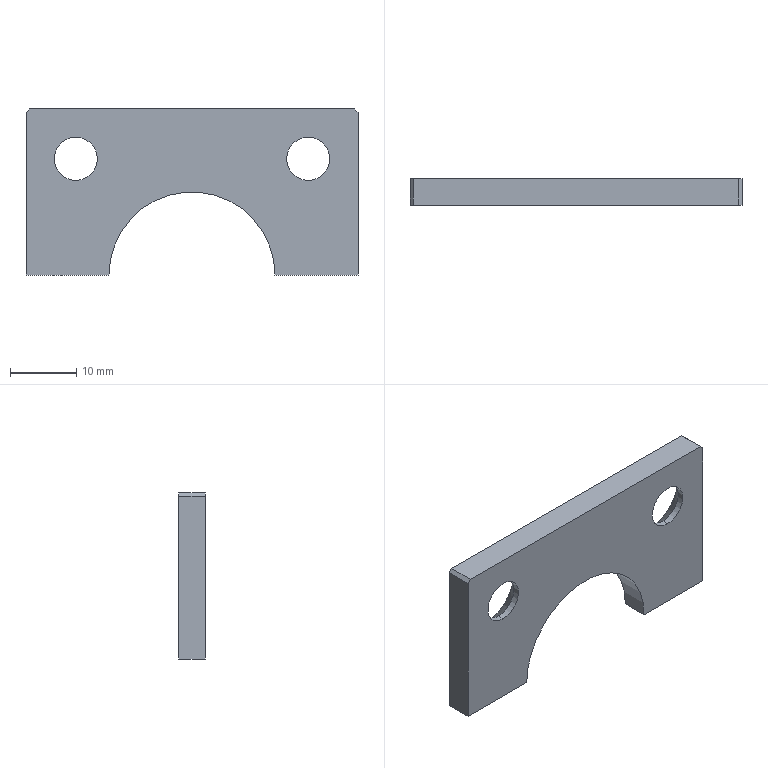Part | STEP file | Cuon T phu H01_4 | 1 solid | 18 faces | box 50 x 4 x 25 mm | volume 3511 mm3 | plane 9 | cylinder 5 | cone 4 | commonest cylinder face diameters 6.5 x4 25 x1
STEP:
#1=CARTESIAN_POINT('',(0.,0.,0.));
#2=DIRECTION('',(0.,0.,1.));
#3=DIRECTION('',(1.,0.,0.));
#4=AXIS2_PLACEMENT_3D('',#1,#2,#3);
#5=CARTESIAN_POINT('',(-17.5,1.,20.75));
#6=VERTEX_POINT('',#5);
#7=CARTESIAN_POINT('',(-17.5,4.,23.75));
#8=VERTEX_POINT('',#7);
#9=CARTESIAN_POINT('',(-17.5,1.,20.75));
#10=DIRECTION('',(0.,0.7071,0.7071));
#11=VECTOR('',#10,1.);
#12=LINE('',#9,#11);
#13=CARTESIAN_POINT('',(-17.5,1.,17.5));
#14=DIRECTION('',(0.,1.,0.));
#15=DIRECTION('',(0.,0.,1.));
#16=AXIS2_PLACEMENT_3D('',#13,#14,#15);
#17=CONICAL_SURFACE('',#16,3.25,0.7854);
#18=CARTESIAN_POINT('',(6.283,0.));
#19=DIRECTION('',(0.,1.));
#20=VECTOR('',#19,1.);
#21=LINE('',#18,#20);
#22=(GEOMETRIC_REPRESENTATION_CONTEXT(2)PARAMETRIC_REPRESENTATION_CONTEXT()REPRESENTATION_CONTEXT('',''));
#23=DEFINITIONAL_REPRESENTATION('',(#21),#22);
#24=PCURVE('',#17,#23);
#25=CARTESIAN_POINT('',(-17.5,1.,17.5));
#26=DIRECTION('',(0.,1.,0.));
#27=DIRECTION('',(0.,0.,1.));
#28=AXIS2_PLACEMENT_3D('',#25,#26,#27);
#29=CONICAL_SURFACE('',#28,3.25,0.7854);
#30=CARTESIAN_POINT('',(0.,0.));
#31=DIRECTION('',(0.,1.));
#32=VECTOR('',#31,1.);
#33=LINE('',#30,#32);
#34=(GEOMETRIC_REPRESENTATION_CONTEXT(2)PARAMETRIC_REPRESENTATION_CONTEXT()REPRESENTATION_CONTEXT('',''));
#35=DEFINITIONAL_REPRESENTATION('',(#33),#34);
#36=PCURVE('',#29,#35);
#37=SURFACE_CURVE('',#12,(#24,#36),.PCURVE_S1.);
#38=EDGE_CURVE('',#6,#8,#37,.T.);
#39=ORIENTED_EDGE('',*,*,#38,.T.);
#40=CARTESIAN_POINT('',(-17.5,4.,11.25));
#41=VERTEX_POINT('',#40);
#42=CARTESIAN_POINT('',(-17.5,4.,17.5));
#43=DIRECTION('',(0.,-1.,0.));
#44=DIRECTION('',(0.,0.,1.));
#45=AXIS2_PLACEMENT_3D('',#42,#43,#44);
#46=CIRCLE('',#45,6.25);
#47=CARTESIAN_POINT('',(6.283,3.));
#48=DIRECTION('',(-1.,0.));
#49=VECTOR('',#48,1.);
#50=LINE('',#47,#49);
#51=(GEOMETRIC_REPRESENTATION_CONTEXT(2)PARAMETRIC_REPRESENTATION_CONTEXT()REPRESENTATION_CONTEXT('',''));
#52=DEFINITIONAL_REPRESENTATION('',(#50),#51);
#53=PCURVE('',#17,#52);
#54=CARTESIAN_POINT('',(0.,4.,0.));
#55=DIRECTION('',(0.,1.,0.));
#56=DIRECTION('',(0.,0.,1.));
#57=AXIS2_PLACEMENT_3D('',#54,#55,#56);
#58=PLANE('',#57);
#59=CARTESIAN_POINT('',(23.75,-17.5));
#60=CARTESIAN_POINT('',(23.75,-28.325));
#61=CARTESIAN_POINT('',(14.375,-22.913));
#62=CARTESIAN_POINT('',(5.,-17.5));
#63=CARTESIAN_POINT('',(14.375,-12.087));
#64=CARTESIAN_POINT('',(23.75,-6.675));
#65=CARTESIAN_POINT('',(23.75,-17.5));
#66=(BOUNDED_CURVE()B_SPLINE_CURVE(2,(#59,#60,#61,#62,#63,#64,#65),.UNSPECIFIED.,.T.,.F.)B_SPLINE_CURVE_WITH_KNOTS((1,2,2,2,2,1),(-2.094,0.,2.094,4.189,6.283,8.378),.UNSPECIFIED.)CURVE()GEOMETRIC_REPRESENTATION_ITEM()RATIONAL_B_SPLINE_CURVE((1.,0.5,1.,0.5,1.,0.5,1.))REPRESENTATION_ITEM(''));
#67=(GEOMETRIC_REPRESENTATION_CONTEXT(2)PARAMETRIC_REPRESENTATION_CONTEXT()REPRESENTATION_CONTEXT('',''));
#68=DEFINITIONAL_REPRESENTATION('',(#66),#67);
#69=PCURVE('',#58,#68);
#70=SURFACE_CURVE('',#46,(#53,#69),.PCURVE_S1.);
#71=EDGE_CURVE('',#8,#41,#70,.T.);
#72=ORIENTED_EDGE('',*,*,#71,.T.);
#73=CARTESIAN_POINT('',(-17.5,1.,14.25));
#74=VERTEX_POINT('',#73);
#75=CARTESIAN_POINT('',(-17.5,1.,14.25));
#76=DIRECTION('',(0.,0.7071,-0.7071));
#77=VECTOR('',#76,1.);
#78=LINE('',#75,#77);
#79=CARTESIAN_POINT('',(3.142,0.));
#80=DIRECTION('',(0.,1.));
#81=VECTOR('',#80,1.);
#82=LINE('',#79,#81);
#83=(GEOMETRIC_REPRESENTATION_CONTEXT(2)PARAMETRIC_REPRESENTATION_CONTEXT()REPRESENTATION_CONTEXT('',''));
#84=DEFINITIONAL_REPRESENTATION('',(#82),#83);
#85=PCURVE('',#17,#84);
#86=CARTESIAN_POINT('',(3.142,0.));
#87=DIRECTION('',(0.,1.));
#88=VECTOR('',#87,1.);
#89=LINE('',#86,#88);
#90=(GEOMETRIC_REPRESENTATION_CONTEXT(2)PARAMETRIC_REPRESENTATION_CONTEXT()REPRESENTATION_CONTEXT('',''));
#91=DEFINITIONAL_REPRESENTATION('',(#89),#90);
#92=PCURVE('',#29,#91);
#93=SURFACE_CURVE('',#78,(#85,#92),.PCURVE_S1.);
#94=EDGE_CURVE('',#74,#41,#93,.T.);
#95=ORIENTED_EDGE('',*,*,#94,.F.);
#96=CARTESIAN_POINT('',(-17.5,1.,17.5));
#97=DIRECTION('',(0.,1.,0.));
#98=DIRECTION('',(0.,0.,1.));
#99=AXIS2_PLACEMENT_3D('',#96,#97,#98);
#100=CIRCLE('',#99,3.25);
#101=CARTESIAN_POINT('',(0.,0.));
#102=DIRECTION('',(1.,0.));
#103=VECTOR('',#102,1.);
#104=LINE('',#101,#103);
#105=(GEOMETRIC_REPRESENTATION_CONTEXT(2)PARAMETRIC_REPRESENTATION_CONTEXT()REPRESENTATION_CONTEXT('',''));
#106=DEFINITIONAL_REPRESENTATION('',(#104),#105);
#107=PCURVE('',#17,#106);
#108=CARTESIAN_POINT('',(-17.5,4.,17.5));
#109=DIRECTION('',(0.,-1.,0.));
#110=DIRECTION('',(0.,0.,-1.));
#111=AXIS2_PLACEMENT_3D('',#108,#109,#110);
#112=CYLINDRICAL_SURFACE('',#111,3.25);
#113=CARTESIAN_POINT('',(9.425,3.));
#114=DIRECTION('',(-1.,0.));
#115=VECTOR('',#114,1.);
#116=LINE('',#113,#115);
#117=(GEOMETRIC_REPRESENTATION_CONTEXT(2)PARAMETRIC_REPRESENTATION_CONTEXT()REPRESENTATION_CONTEXT('',''));
#118=DEFINITIONAL_REPRESENTATION('',(#116),#117);
#119=PCURVE('',#112,#118);
#120=SURFACE_CURVE('',#100,(#107,#119),.PCURVE_S1.);
#121=EDGE_CURVE('',#74,#6,#120,.T.);
#122=ORIENTED_EDGE('',*,*,#121,.T.);
#123=EDGE_LOOP('',(#39,#72,#95,#122));
#124=FACE_BOUND('',#123,.F.);
#125=ADVANCED_FACE('',(#124),#17,.F.);
#126=CARTESIAN_POINT('',(17.5,1.,20.75));
#127=VERTEX_POINT('',#126);
#128=CARTESIAN_POINT('',(17.5,4.,23.75));
#129=VERTEX_POINT('',#128);
#130=CARTESIAN_POINT('',(17.5,1.,20.75));
#131=DIRECTION('',(0.,0.7071,0.7071));
#132=VECTOR('',#131,1.);
#133=LINE('',#130,#132);
#134=CARTESIAN_POINT('',(17.5,1.,17.5));
#135=DIRECTION('',(0.,1.,0.));
#136=DIRECTION('',(0.,0.,1.));
#137=AXIS2_PLACEMENT_3D('',#134,#135,#136);
#138=CONICAL_SURFACE('',#137,3.25,0.7854);
#139=CARTESIAN_POINT('',(6.283,0.));
#140=DIRECTION('',(0.,1.));
#141=VECTOR('',#140,1.);
#142=LINE('',#139,#141);
#143=(GEOMETRIC_REPRESENTATION_CONTEXT(2)PARAMETRIC_REPRESENTATION_CONTEXT()REPRESENTATION_CONTEXT('',''));
#144=DEFINITIONAL_REPRESENTATION('',(#142),#143);
#145=PCURVE('',#138,#144);
#146=CARTESIAN_POINT('',(17.5,1.,17.5));
#147=DIRECTION('',(0.,1.,0.));
#148=DIRECTION('',(0.,0.,1.));
#149=AXIS2_PLACEMENT_3D('',#146,#147,#148);
#150=CONICAL_SURFACE('',#149,3.25,0.7854);
#151=CARTESIAN_POINT('',(0.,0.));
#152=DIRECTION('',(0.,1.));
#153=VECTOR('',#152,1.);
#154=LINE('',#151,#153);
#155=(GEOMETRIC_REPRESENTATION_CONTEXT(2)PARAMETRIC_REPRESENTATION_CONTEXT()REPRESENTATION_CONTEXT('',''));
#156=DEFINITIONAL_REPRESENTATION('',(#154),#155);
#157=PCURVE('',#150,#156);
#158=SURFACE_CURVE('',#133,(#145,#157),.PCURVE_S1.);
#159=EDGE_CURVE('',#127,#129,#158,.T.);
#160=ORIENTED_EDGE('',*,*,#159,.T.);
#161=CARTESIAN_POINT('',(17.5,4.,11.25));
#162=VERTEX_POINT('',#161);
#163=CARTESIAN_POINT('',(17.5,4.,17.5));
#164=DIRECTION('',(0.,-1.,0.));
#165=DIRECTION('',(0.,0.,1.));
#166=AXIS2_PLACEMENT_3D('',#163,#164,#165);
#167=CIRCLE('',#166,6.25);
#168=CARTESIAN_POINT('',(6.283,3.));
#169=DIRECTION('',(-1.,0.));
#170=VECTOR('',#169,1.);
#171=LINE('',#168,#170);
#172=(GEOMETRIC_REPRESENTATION_CONTEXT(2)PARAMETRIC_REPRESENTATION_CONTEXT()REPRESENTATION_CONTEXT('',''));
#173=DEFINITIONAL_REPRESENTATION('',(#171),#172);
#174=PCURVE('',#138,#173);
#175=CARTESIAN_POINT('',(23.75,17.5));
#176=CARTESIAN_POINT('',(23.75,6.675));
#177=CARTESIAN_POINT('',(14.375,12.087));
#178=CARTESIAN_POINT('',(5.,17.5));
#179=CARTESIAN_POINT('',(14.375,22.913));
#180=CARTESIAN_POINT('',(23.75,28.325));
#181=CARTESIAN_POINT('',(23.75,17.5));
#182=(BOUNDED_CURVE()B_SPLINE_CURVE(2,(#175,#176,#177,#178,#179,#180,#181),.UNSPECIFIED.,.T.,.F.)B_SPLINE_CURVE_WITH_KNOTS((1,2,2,2,2,1),(-2.094,0.,2.094,4.189,6.283,8.378),.UNSPECIFIED.)CURVE()GEOMETRIC_REPRESENTATION_ITEM()RATIONAL_B_SPLINE_CURVE((1.,0.5,1.,0.5,1.,0.5,1.))REPRESENTATION_ITEM(''));
#183=(GEOMETRIC_REPRESENTATION_CONTEXT(2)PARAMETRIC_REPRESENTATION_CONTEXT()REPRESENTATION_CONTEXT('',''));
#184=DEFINITIONAL_REPRESENTATION('',(#182),#183);
#185=PCURVE('',#58,#184);
#186=SURFACE_CURVE('',#167,(#174,#185),.PCURVE_S1.);
#187=EDGE_CURVE('',#129,#162,#186,.T.);
#188=ORIENTED_EDGE('',*,*,#187,.T.);
#189=CARTESIAN_POINT('',(17.5,1.,14.25));
#190=VERTEX_POINT('',#189);
#191=CARTESIAN_POINT('',(17.5,1.,14.25));
#192=DIRECTION('',(0.,0.7071,-0.7071));
#193=VECTOR('',#192,1.);
#194=LINE('',#191,#193);
#195=CARTESIAN_POINT('',(3.142,0.));
#196=DIRECTION('',(0.,1.));
#197=VECTOR('',#196,1.);
#198=LINE('',#195,#197);
#199=(GEOMETRIC_REPRESENTATION_CONTEXT(2)PARAMETRIC_REPRESENTATION_CONTEXT()REPRESENTATION_CONTEXT('',''));
#200=DEFINITIONAL_REPRESENTATION('',(#198),#199);
#201=PCURVE('',#138,#200);
#202=CARTESIAN_POINT('',(3.142,0.));
#203=DIRECTION('',(0.,1.));
#204=VECTOR('',#203,1.);
#205=LINE('',#202,#204);
#206=(GEOMETRIC_REPRESENTATION_CONTEXT(2)PARAMETRIC_REPRESENTATION_CONTEXT()REPRESENTATION_CONTEXT('',''));
#207=DEFINITIONAL_REPRESENTATION('',(#205),#206);
#208=PCURVE('',#150,#207);
#209=SURFACE_CURVE('',#194,(#201,#208),.PCURVE_S1.);
#210=EDGE_CURVE('',#190,#162,#209,.T.);
#211=ORIENTED_EDGE('',*,*,#210,.F.);
#212=CARTESIAN_POINT('',(17.5,1.,17.5));
#213=DIRECTION('',(0.,1.,0.));
#214=DIRECTION('',(0.,0.,1.));
#215=AXIS2_PLACEMENT_3D('',#212,#213,#214);
#216=CIRCLE('',#215,3.25);
#217=CARTESIAN_POINT('',(0.,0.));
#218=DIRECTION('',(1.,0.));
#219=VECTOR('',#218,1.);
#220=LINE('',#217,#219);
#221=(GEOMETRIC_REPRESENTATION_CONTEXT(2)PARAMETRIC_REPRESENTATION_CONTEXT()REPRESENTATION_CONTEXT('',''));
#222=DEFINITIONAL_REPRESENTATION('',(#220),#221);
#223=PCURVE('',#138,#222);
#224=CARTESIAN_POINT('',(17.5,4.,17.5));
#225=DIRECTION('',(0.,-1.,0.));
#226=DIRECTION('',(0.,0.,-1.));
#227=AXIS2_PLACEMENT_3D('',#224,#225,#226);
#228=CYLINDRICAL_SURFACE('',#227,3.25);
#229=CARTESIAN_POINT('',(9.425,3.));
#230=DIRECTION('',(-1.,0.));
#231=VECTOR('',#230,1.);
#232=LINE('',#229,#231);
#233=(GEOMETRIC_REPRESENTATION_CONTEXT(2)PARAMETRIC_REPRESENTATION_CONTEXT()REPRESENTATION_CONTEXT('',''));
#234=DEFINITIONAL_REPRESENTATION('',(#232),#233);
#235=PCURVE('',#228,#234);
#236=SURFACE_CURVE('',#216,(#223,#235),.PCURVE_S1.);
#237=EDGE_CURVE('',#190,#127,#236,.T.);
#238=ORIENTED_EDGE('',*,*,#237,.T.);
#239=EDGE_LOOP('',(#160,#188,#211,#238));
#240=FACE_BOUND('',#239,.F.);
#241=ADVANCED_FACE('',(#240),#138,.F.);
#242=CARTESIAN_POINT('',(-17.5,0.,14.25));
#243=VERTEX_POINT('',#242);
#244=CARTESIAN_POINT('',(-17.5,4.,14.25));
#245=DIRECTION('',(0.,-1.,0.));
#246=VECTOR('',#245,1.);
#247=LINE('',#244,#246);
#248=CARTESIAN_POINT('',(6.283,0.));
#249=DIRECTION('',(0.,1.));
#250=VECTOR('',#249,1.);
#251=LINE('',#248,#250);
#252=(GEOMETRIC_REPRESENTATION_CONTEXT(2)PARAMETRIC_REPRESENTATION_CONTEXT()REPRESENTATION_CONTEXT('',''));
#253=DEFINITIONAL_REPRESENTATION('',(#251),#252);
#254=PCURVE('',#112,#253);
#255=CARTESIAN_POINT('',(-17.5,4.,17.5));
#256=DIRECTION('',(0.,-1.,0.));
#257=DIRECTION('',(0.,0.,-1.));
#258=AXIS2_PLACEMENT_3D('',#255,#256,#257);
#259=CYLINDRICAL_SURFACE('',#258,3.25);
#260=CARTESIAN_POINT('',(0.,0.));
#261=DIRECTION('',(0.,1.));
#262=VECTOR('',#261,1.);
#263=LINE('',#260,#262);
#264=(GEOMETRIC_REPRESENTATION_CONTEXT(2)PARAMETRIC_REPRESENTATION_CONTEXT()REPRESENTATION_CONTEXT('',''));
#265=DEFINITIONAL_REPRESENTATION('',(#263),#264);
#266=PCURVE('',#259,#265);
#267=SURFACE_CURVE('',#247,(#254,#266),.PCURVE_S1.);
#268=EDGE_CURVE('',#74,#243,#267,.T.);
#269=ORIENTED_EDGE('',*,*,#268,.T.);
#270=CARTESIAN_POINT('',(-17.5,0.,20.75));
#271=VERTEX_POINT('',#270);
#272=CARTESIAN_POINT('',(-17.5,0.,17.5));
#273=DIRECTION('',(0.,1.,0.));
#274=DIRECTION('',(0.,0.,1.));
#275=AXIS2_PLACEMENT_3D('',#272,#273,#274);
#276=CIRCLE('',#275,3.25);
#277=CARTESIAN_POINT('',(9.425,4.));
#278=DIRECTION('',(-1.,0.));
#279=VECTOR('',#278,1.);
#280=LINE('',#277,#279);
#281=(GEOMETRIC_REPRESENTATION_CONTEXT(2)PARAMETRIC_REPRESENTATION_CONTEXT()REPRESENTATION_CONTEXT('',''));
#282=DEFINITIONAL_REPRESENTATION('',(#280),#281);
#283=PCURVE('',#112,#282);
#284=CARTESIAN_POINT('',(0.,0.,0.));
#285=DIRECTION('',(0.,1.,0.));
#286=DIRECTION('',(0.,0.,1.));
#287=AXIS2_PLACEMENT_3D('',#284,#285,#286);
#288=PLANE('',#287);
#289=CARTESIAN_POINT('',(17.5,-17.5));
#290=DIRECTION('',(1.,0.));
#291=AXIS2_PLACEMENT_2D('',#289,#290);
#292=CIRCLE('',#291,3.25);
#293=(GEOMETRIC_REPRESENTATION_CONTEXT(2)PARAMETRIC_REPRESENTATION_CONTEXT()REPRESENTATION_CONTEXT('',''));
#294=DEFINITIONAL_REPRESENTATION('',(#292),#293);
#295=PCURVE('',#288,#294);
#296=SURFACE_CURVE('',#276,(#283,#295),.PCURVE_S1.);
#297=EDGE_CURVE('',#243,#271,#296,.T.);
#298=ORIENTED_EDGE('',*,*,#297,.T.);
#299=CARTESIAN_POINT('',(-17.5,4.,20.75));
#300=DIRECTION('',(0.,-1.,0.));
#301=VECTOR('',#300,1.);
#302=LINE('',#299,#301);
#303=CARTESIAN_POINT('',(3.142,0.));
#304=DIRECTION('',(0.,1.));
#305=VECTOR('',#304,1.);
#306=LINE('',#303,#305);
#307=(GEOMETRIC_REPRESENTATION_CONTEXT(2)PARAMETRIC_REPRESENTATION_CONTEXT()REPRESENTATION_CONTEXT('',''));
#308=DEFINITIONAL_REPRESENTATION('',(#306),#307);
#309=PCURVE('',#112,#308);
#310=CARTESIAN_POINT('',(3.142,0.));
#311=DIRECTION('',(0.,1.));
#312=VECTOR('',#311,1.);
#313=LINE('',#310,#312);
#314=(GEOMETRIC_REPRESENTATION_CONTEXT(2)PARAMETRIC_REPRESENTATION_CONTEXT()REPRESENTATION_CONTEXT('',''));
#315=DEFINITIONAL_REPRESENTATION('',(#313),#314);
#316=PCURVE('',#259,#315);
#317=SURFACE_CURVE('',#302,(#309,#316),.PCURVE_S1.);
#318=EDGE_CURVE('',#6,#271,#317,.T.);
#319=ORIENTED_EDGE('',*,*,#318,.F.);
#320=ORIENTED_EDGE('',*,*,#121,.F.);
#321=EDGE_LOOP('',(#269,#298,#319,#320));
#322=FACE_BOUND('',#321,.F.);
#323=ADVANCED_FACE('',(#322),#112,.F.);
#324=CARTESIAN_POINT('',(17.5,0.,14.25));
#325=VERTEX_POINT('',#324);
#326=CARTESIAN_POINT('',(17.5,4.,14.25));
#327=DIRECTION('',(0.,-1.,0.));
#328=VECTOR('',#327,1.);
#329=LINE('',#326,#328);
#330=CARTESIAN_POINT('',(6.283,0.));
#331=DIRECTION('',(0.,1.));
#332=VECTOR('',#331,1.);
#333=LINE('',#330,#332);
#334=(GEOMETRIC_REPRESENTATION_CONTEXT(2)PARAMETRIC_REPRESENTATION_CONTEXT()REPRESENTATION_CONTEXT('',''));
#335=DEFINITIONAL_REPRESENTATION('',(#333),#334);
#336=PCURVE('',#228,#335);
#337=CARTESIAN_POINT('',(17.5,4.,17.5));
#338=DIRECTION('',(0.,-1.,0.));
#339=DIRECTION('',(0.,0.,-1.));
#340=AXIS2_PLACEMENT_3D('',#337,#338,#339);
#341=CYLINDRICAL_SURFACE('',#340,3.25);
#342=CARTESIAN_POINT('',(0.,0.));
#343=DIRECTION('',(0.,1.));
#344=VECTOR('',#343,1.);
#345=LINE('',#342,#344);
#346=(GEOMETRIC_REPRESENTATION_CONTEXT(2)PARAMETRIC_REPRESENTATION_CONTEXT()REPRESENTATION_CONTEXT('',''));
#347=DEFINITIONAL_REPRESENTATION('',(#345),#346);
#348=PCURVE('',#341,#347);
#349=SURFACE_CURVE('',#329,(#336,#348),.PCURVE_S1.);
#350=EDGE_CURVE('',#190,#325,#349,.T.);
#351=ORIENTED_EDGE('',*,*,#350,.T.);
#352=CARTESIAN_POINT('',(17.5,0.,20.75));
#353=VERTEX_POINT('',#352);
#354=CARTESIAN_POINT('',(17.5,0.,17.5));
#355=DIRECTION('',(0.,1.,0.));
#356=DIRECTION('',(0.,0.,1.));
#357=AXIS2_PLACEMENT_3D('',#354,#355,#356);
#358=CIRCLE('',#357,3.25);
#359=CARTESIAN_POINT('',(9.425,4.));
#360=DIRECTION('',(-1.,0.));
#361=VECTOR('',#360,1.);
#362=LINE('',#359,#361);
#363=(GEOMETRIC_REPRESENTATION_CONTEXT(2)PARAMETRIC_REPRESENTATION_CONTEXT()REPRESENTATION_CONTEXT('',''));
#364=DEFINITIONAL_REPRESENTATION('',(#362),#363);
#365=PCURVE('',#228,#364);
#366=CARTESIAN_POINT('',(17.5,17.5));
#367=DIRECTION('',(1.,0.));
#368=AXIS2_PLACEMENT_2D('',#366,#367);
#369=CIRCLE('',#368,3.25);
#370=(GEOMETRIC_REPRESENTATION_CONTEXT(2)PARAMETRIC_REPRESENTATION_CONTEXT()REPRESENTATION_CONTEXT('',''));
#371=DEFINITIONAL_REPRESENTATION('',(#369),#370);
#372=PCURVE('',#288,#371);
#373=SURFACE_CURVE('',#358,(#365,#372),.PCURVE_S1.);
#374=EDGE_CURVE('',#325,#353,#373,.T.);
#375=ORIENTED_EDGE('',*,*,#374,.T.);
#376=CARTESIAN_POINT('',(17.5,4.,20.75));
#377=DIRECTION('',(0.,-1.,0.));
#378=VECTOR('',#377,1.);
#379=LINE('',#376,#378);
#380=CARTESIAN_POINT('',(3.142,0.));
#381=DIRECTION('',(0.,1.));
#382=VECTOR('',#381,1.);
#383=LINE('',#380,#382);
#384=(GEOMETRIC_REPRESENTATION_CONTEXT(2)PARAMETRIC_REPRESENTATION_CONTEXT()REPRESENTATION_CONTEXT('',''));
#385=DEFINITIONAL_REPRESENTATION('',(#383),#384);
#386=PCURVE('',#228,#385);
#387=CARTESIAN_POINT('',(3.142,0.));
#388=DIRECTION('',(0.,1.));
#389=VECTOR('',#388,1.);
#390=LINE('',#387,#389);
#391=(GEOMETRIC_REPRESENTATION_CONTEXT(2)PARAMETRIC_REPRESENTATION_CONTEXT()REPRESENTATION_CONTEXT('',''));
#392=DEFINITIONAL_REPRESENTATION('',(#390),#391);
#393=PCURVE('',#341,#392);
#394=SURFACE_CURVE('',#379,(#386,#393),.PCURVE_S1.);
#395=EDGE_CURVE('',#127,#353,#394,.T.);
#396=ORIENTED_EDGE('',*,*,#395,.F.);
#397=ORIENTED_EDGE('',*,*,#237,.F.);
#398=EDGE_LOOP('',(#351,#375,#396,#397));
#399=FACE_BOUND('',#398,.F.);
#400=ADVANCED_FACE('',(#399),#228,.F.);
#401=CARTESIAN_POINT('',(-25.,4.,0.));
#402=VERTEX_POINT('',#401);
#403=CARTESIAN_POINT('',(-12.5,4.,0.));
#404=VERTEX_POINT('',#403);
#405=CARTESIAN_POINT('',(0.,4.,0.));
#406=DIRECTION('',(1.,0.,0.));
#407=VECTOR('',#406,1.);
#408=LINE('',#405,#407);
#409=CARTESIAN_POINT('',(0.,0.));
#410=DIRECTION('',(0.,1.));
#411=VECTOR('',#410,1.);
#412=LINE('',#409,#411);
#413=(GEOMETRIC_REPRESENTATION_CONTEXT(2)PARAMETRIC_REPRESENTATION_CONTEXT()REPRESENTATION_CONTEXT('',''));
#414=DEFINITIONAL_REPRESENTATION('',(#412),#413);
#415=PCURVE('',#58,#414);
#416=CARTESIAN_POINT('',(-120.,45.57,0.));
#417=DIRECTION('',(0.,0.,1.));
#418=DIRECTION('',(-1.,0.,0.));
#419=AXIS2_PLACEMENT_3D('',#416,#417,#418);
#420=PLANE('',#419);
#421=CARTESIAN_POINT('',(-120.,41.57));
#422=DIRECTION('',(-1.,0.));
#423=VECTOR('',#422,1.);
#424=LINE('',#421,#423);
#425=(GEOMETRIC_REPRESENTATION_CONTEXT(2)PARAMETRIC_REPRESENTATION_CONTEXT()REPRESENTATION_CONTEXT('',''));
#426=DEFINITIONAL_REPRESENTATION('',(#424),#425);
#427=PCURVE('',#420,#426);
#428=SURFACE_CURVE('',#408,(#415,#427),.PCURVE_S1.);
#429=EDGE_CURVE('',#402,#404,#428,.T.);
#430=ORIENTED_EDGE('',*,*,#429,.F.);
#431=CARTESIAN_POINT('',(-25.,4.,24.5));
#432=VERTEX_POINT('',#431);
#433=CARTESIAN_POINT('',(-25.,4.,-25.));
#434=DIRECTION('',(0.,0.,1.));
#435=VECTOR('',#434,1.);
#436=LINE('',#433,#435);
#437=CARTESIAN_POINT('',(-25.,-25.));
#438=DIRECTION('',(1.,0.));
#439=VECTOR('',#438,1.);
#440=LINE('',#437,#439);
#441=(GEOMETRIC_REPRESENTATION_CONTEXT(2)PARAMETRIC_REPRESENTATION_CONTEXT()REPRESENTATION_CONTEXT('',''));
#442=DEFINITIONAL_REPRESENTATION('',(#440),#441);
#443=PCURVE('',#58,#442);
#444=CARTESIAN_POINT('',(-25.,4.,-25.));
#445=DIRECTION('',(1.,0.,0.));
#446=DIRECTION('',(0.,0.,-1.));
#447=AXIS2_PLACEMENT_3D('',#444,#445,#446);
#448=PLANE('',#447);
#449=CARTESIAN_POINT('',(0.,0.));
#450=DIRECTION('',(-1.,0.));
#451=VECTOR('',#450,1.);
#452=LINE('',#449,#451);
#453=(GEOMETRIC_REPRESENTATION_CONTEXT(2)PARAMETRIC_REPRESENTATION_CONTEXT()REPRESENTATION_CONTEXT('',''));
#454=DEFINITIONAL_REPRESENTATION('',(#452),#453);
#455=PCURVE('',#448,#454);
#456=SURFACE_CURVE('',#436,(#443,#455),.PCURVE_S1.);
#457=EDGE_CURVE('',#402,#432,#456,.T.);
#458=ORIENTED_EDGE('',*,*,#457,.T.);
#459=CARTESIAN_POINT('',(-24.5,4.,25.));
#460=VERTEX_POINT('',#459);
#461=CARTESIAN_POINT('',(-24.75,4.,24.75));
#462=DIRECTION('',(0.7071,0.,0.7071));
#463=VECTOR('',#462,1.);
#464=LINE('',#461,#463);
#465=CARTESIAN_POINT('',(24.75,-24.75));
#466=DIRECTION('',(0.7071,0.7071));
#467=VECTOR('',#466,1.);
#468=LINE('',#465,#467);
#469=(GEOMETRIC_REPRESENTATION_CONTEXT(2)PARAMETRIC_REPRESENTATION_CONTEXT()REPRESENTATION_CONTEXT('',''));
#470=DEFINITIONAL_REPRESENTATION('',(#468),#469);
#471=PCURVE('',#58,#470);
#472=CARTESIAN_POINT('',(-24.5,4.,25.));
#473=DIRECTION('',(0.7071,0.,-0.7071));
#474=DIRECTION('',(0.,-1.,0.));
#475=AXIS2_PLACEMENT_3D('',#472,#473,#474);
#476=PLANE('',#475);
#477=CARTESIAN_POINT('',(0.,0.3536));
#478=DIRECTION('',(0.,-1.));
#479=VECTOR('',#478,1.);
#480=LINE('',#477,#479);
#481=(GEOMETRIC_REPRESENTATION_CONTEXT(2)PARAMETRIC_REPRESENTATION_CONTEXT()REPRESENTATION_CONTEXT('',''));
#482=DEFINITIONAL_REPRESENTATION('',(#480),#481);
#483=PCURVE('',#476,#482);
#484=SURFACE_CURVE('',#464,(#471,#483),.PCURVE_S1.);
#485=EDGE_CURVE('',#432,#460,#484,.T.);
#486=ORIENTED_EDGE('',*,*,#485,.T.);
#487=CARTESIAN_POINT('',(24.5,4.,25.));
#488=VERTEX_POINT('',#487);
#489=CARTESIAN_POINT('',(-25.,4.,25.));
#490=DIRECTION('',(1.,0.,0.));
#491=VECTOR('',#490,1.);
#492=LINE('',#489,#491);
#493=CARTESIAN_POINT('',(25.,-25.));
#494=DIRECTION('',(0.,1.));
#495=VECTOR('',#494,1.);
#496=LINE('',#493,#495);
#497=(GEOMETRIC_REPRESENTATION_CONTEXT(2)PARAMETRIC_REPRESENTATION_CONTEXT()REPRESENTATION_CONTEXT('',''));
#498=DEFINITIONAL_REPRESENTATION('',(#496),#497);
#499=PCURVE('',#58,#498);
#500=CARTESIAN_POINT('',(-25.,4.,25.));
#501=DIRECTION('',(0.,0.,-1.));
#502=DIRECTION('',(-1.,0.,0.));
#503=AXIS2_PLACEMENT_3D('',#500,#501,#502);
#504=PLANE('',#503);
#505=CARTESIAN_POINT('',(0.,0.));
#506=DIRECTION('',(-1.,0.));
#507=VECTOR('',#506,1.);
#508=LINE('',#505,#507);
#509=(GEOMETRIC_REPRESENTATION_CONTEXT(2)PARAMETRIC_REPRESENTATION_CONTEXT()REPRESENTATION_CONTEXT('',''));
#510=DEFINITIONAL_REPRESENTATION('',(#508),#509);
#511=PCURVE('',#504,#510);
#512=SURFACE_CURVE('',#492,(#499,#511),.PCURVE_S1.);
#513=EDGE_CURVE('',#460,#488,#512,.T.);
#514=ORIENTED_EDGE('',*,*,#513,.T.);
#515=CARTESIAN_POINT('',(25.,4.,24.5));
#516=VERTEX_POINT('',#515);
#517=CARTESIAN_POINT('',(24.75,4.,24.75));
#518=DIRECTION('',(0.7071,0.,-0.7071));
#519=VECTOR('',#518,1.);
#520=LINE('',#517,#519);
#521=CARTESIAN_POINT('',(24.75,24.75));
#522=DIRECTION('',(-0.7071,0.7071));
#523=VECTOR('',#522,1.);
#524=LINE('',#521,#523);
#525=(GEOMETRIC_REPRESENTATION_CONTEXT(2)PARAMETRIC_REPRESENTATION_CONTEXT()REPRESENTATION_CONTEXT('',''));
#526=DEFINITIONAL_REPRESENTATION('',(#524),#525);
#527=PCURVE('',#58,#526);
#528=CARTESIAN_POINT('',(25.,4.,24.5));
#529=DIRECTION('',(-0.7071,0.,-0.7071));
#530=DIRECTION('',(0.,-1.,0.));
#531=AXIS2_PLACEMENT_3D('',#528,#529,#530);
#532=PLANE('',#531);
#533=CARTESIAN_POINT('',(0.,0.3536));
#534=DIRECTION('',(0.,-1.));
#535=VECTOR('',#534,1.);
#536=LINE('',#533,#535);
#537=(GEOMETRIC_REPRESENTATION_CONTEXT(2)PARAMETRIC_REPRESENTATION_CONTEXT()REPRESENTATION_CONTEXT('',''));
#538=DEFINITIONAL_REPRESENTATION('',(#536),#537);
#539=PCURVE('',#532,#538);
#540=SURFACE_CURVE('',#520,(#527,#539),.PCURVE_S1.);
#541=EDGE_CURVE('',#488,#516,#540,.T.);
#542=ORIENTED_EDGE('',*,*,#541,.T.);
#543=CARTESIAN_POINT('',(25.,4.,0.));
#544=VERTEX_POINT('',#543);
#545=CARTESIAN_POINT('',(25.,4.,-25.));
#546=DIRECTION('',(0.,0.,-1.));
#547=VECTOR('',#546,1.);
#548=LINE('',#545,#547);
#549=CARTESIAN_POINT('',(-25.,25.));
#550=DIRECTION('',(-1.,0.));
#551=VECTOR('',#550,1.);
#552=LINE('',#549,#551);
#553=(GEOMETRIC_REPRESENTATION_CONTEXT(2)PARAMETRIC_REPRESENTATION_CONTEXT()REPRESENTATION_CONTEXT('',''));
#554=DEFINITIONAL_REPRESENTATION('',(#552),#553);
#555=PCURVE('',#58,#554);
#556=CARTESIAN_POINT('',(25.,4.,-25.));
#557=DIRECTION('',(-1.,0.,0.));
#558=DIRECTION('',(0.,0.,1.));
#559=AXIS2_PLACEMENT_3D('',#556,#557,#558);
#560=PLANE('',#559);
#561=CARTESIAN_POINT('',(0.,0.));
#562=DIRECTION('',(-1.,0.));
#563=VECTOR('',#562,1.);
#564=LINE('',#561,#563);
#565=(GEOMETRIC_REPRESENTATION_CONTEXT(2)PARAMETRIC_REPRESENTATION_CONTEXT()REPRESENTATION_CONTEXT('',''));
#566=DEFINITIONAL_REPRESENTATION('',(#564),#565);
#567=PCURVE('',#560,#566);
#568=SURFACE_CURVE('',#548,(#555,#567),.PCURVE_S1.);
#569=EDGE_CURVE('',#516,#544,#568,.T.);
#570=ORIENTED_EDGE('',*,*,#569,.T.);
#571=CARTESIAN_POINT('',(12.5,4.,0.));
#572=VERTEX_POINT('',#571);
#573=CARTESIAN_POINT('',(0.,4.,0.));
#574=DIRECTION('',(1.,0.,0.));
#575=VECTOR('',#574,1.);
#576=LINE('',#573,#575);
#577=CARTESIAN_POINT('',(0.,0.));
#578=DIRECTION('',(0.,1.));
#579=VECTOR('',#578,1.);
#580=LINE('',#577,#579);
#581=(GEOMETRIC_REPRESENTATION_CONTEXT(2)PARAMETRIC_REPRESENTATION_CONTEXT()REPRESENTATION_CONTEXT('',''));
#582=DEFINITIONAL_REPRESENTATION('',(#580),#581);
#583=PCURVE('',#58,#582);
#584=CARTESIAN_POINT('',(-120.,45.57,0.));
#585=DIRECTION('',(0.,0.,1.));
#586=DIRECTION('',(-1.,0.,0.));
#587=AXIS2_PLACEMENT_3D('',#584,#585,#586);
#588=PLANE('',#587);
#589=CARTESIAN_POINT('',(-120.,41.57));
#590=DIRECTION('',(-1.,0.));
#591=VECTOR('',#590,1.);
#592=LINE('',#589,#591);
#593=(GEOMETRIC_REPRESENTATION_CONTEXT(2)PARAMETRIC_REPRESENTATION_CONTEXT()REPRESENTATION_CONTEXT('',''));
#594=DEFINITIONAL_REPRESENTATION('',(#592),#593);
#595=PCURVE('',#588,#594);
#596=SURFACE_CURVE('',#576,(#583,#595),.PCURVE_S1.);
#597=EDGE_CURVE('',#572,#544,#596,.T.);
#598=ORIENTED_EDGE('',*,*,#597,.F.);
#599=CARTESIAN_POINT('',(0.,4.,0.));
#600=DIRECTION('',(0.,1.,0.));
#601=DIRECTION('',(0.,0.,1.));
#602=AXIS2_PLACEMENT_3D('',#599,#600,#601);
#603=CIRCLE('',#602,12.5);
#604=CARTESIAN_POINT('',(0.,0.));
#605=DIRECTION('',(1.,0.));
#606=AXIS2_PLACEMENT_2D('',#604,#605);
#607=CIRCLE('',#606,12.5);
#608=(GEOMETRIC_REPRESENTATION_CONTEXT(2)PARAMETRIC_REPRESENTATION_CONTEXT()REPRESENTATION_CONTEXT('',''));
#609=DEFINITIONAL_REPRESENTATION('',(#607),#608);
#610=PCURVE('',#58,#609);
#611=CARTESIAN_POINT('',(0.,4.,0.));
#612=DIRECTION('',(0.,-1.,0.));
#613=DIRECTION('',(0.,0.,-1.));
#614=AXIS2_PLACEMENT_3D('',#611,#612,#613);
#615=CYLINDRICAL_SURFACE('',#614,12.5);
#616=CARTESIAN_POINT('',(9.425,0.));
#617=DIRECTION('',(-1.,0.));
#618=VECTOR('',#617,1.);
#619=LINE('',#616,#618);
#620=(GEOMETRIC_REPRESENTATION_CONTEXT(2)PARAMETRIC_REPRESENTATION_CONTEXT()REPRESENTATION_CONTEXT('',''));
#621=DEFINITIONAL_REPRESENTATION('',(#619),#620);
#622=PCURVE('',#615,#621);
#623=SURFACE_CURVE('',#603,(#610,#622),.PCURVE_S1.);
#624=EDGE_CURVE('',#404,#572,#623,.T.);
#625=ORIENTED_EDGE('',*,*,#624,.F.);
#626=EDGE_LOOP('',(#430,#458,#486,#514,#542,#570,#598,#625));
#627=FACE_BOUND('',#626,.T.);
#628=ORIENTED_EDGE('',*,*,#187,.T.);
#629=CARTESIAN_POINT('',(17.5,4.,17.5));
#630=DIRECTION('',(0.,-1.,0.));
#631=DIRECTION('',(0.,0.,1.));
#632=AXIS2_PLACEMENT_3D('',#629,#630,#631);
#633=CIRCLE('',#632,6.25);
#634=CARTESIAN_POINT('',(23.75,17.5));
#635=CARTESIAN_POINT('',(23.75,6.675));
#636=CARTESIAN_POINT('',(14.375,12.087));
#637=CARTESIAN_POINT('',(5.,17.5));
#638=CARTESIAN_POINT('',(14.375,22.913));
#639=CARTESIAN_POINT('',(23.75,28.325));
#640=CARTESIAN_POINT('',(23.75,17.5));
#641=(BOUNDED_CURVE()B_SPLINE_CURVE(2,(#634,#635,#636,#637,#638,#639,#640),.UNSPECIFIED.,.T.,.F.)B_SPLINE_CURVE_WITH_KNOTS((1,2,2,2,2,1),(-2.094,0.,2.094,4.189,6.283,8.378),.UNSPECIFIED.)CURVE()GEOMETRIC_REPRESENTATION_ITEM()RATIONAL_B_SPLINE_CURVE((1.,0.5,1.,0.5,1.,0.5,1.))REPRESENTATION_ITEM(''));
#642=(GEOMETRIC_REPRESENTATION_CONTEXT(2)PARAMETRIC_REPRESENTATION_CONTEXT()REPRESENTATION_CONTEXT('',''));
#643=DEFINITIONAL_REPRESENTATION('',(#641),#642);
#644=PCURVE('',#58,#643);
#645=CARTESIAN_POINT('',(6.283,3.));
#646=DIRECTION('',(-1.,0.));
#647=VECTOR('',#646,1.);
#648=LINE('',#645,#647);
#649=(GEOMETRIC_REPRESENTATION_CONTEXT(2)PARAMETRIC_REPRESENTATION_CONTEXT()REPRESENTATION_CONTEXT('',''));
#650=DEFINITIONAL_REPRESENTATION('',(#648),#649);
#651=PCURVE('',#150,#650);
#652=SURFACE_CURVE('',#633,(#644,#651),.PCURVE_S1.);
#653=EDGE_CURVE('',#162,#129,#652,.T.);
#654=ORIENTED_EDGE('',*,*,#653,.T.);
#655=EDGE_LOOP('',(#628,#654));
#656=FACE_BOUND('',#655,.T.);
#657=ORIENTED_EDGE('',*,*,#71,.T.);
#658=CARTESIAN_POINT('',(-17.5,4.,17.5));
#659=DIRECTION('',(0.,-1.,0.));
#660=DIRECTION('',(0.,0.,1.));
#661=AXIS2_PLACEMENT_3D('',#658,#659,#660);
#662=CIRCLE('',#661,6.25);
#663=CARTESIAN_POINT('',(23.75,-17.5));
#664=CARTESIAN_POINT('',(23.75,-28.325));
#665=CARTESIAN_POINT('',(14.375,-22.913));
#666=CARTESIAN_POINT('',(5.,-17.5));
#667=CARTESIAN_POINT('',(14.375,-12.087));
#668=CARTESIAN_POINT('',(23.75,-6.675));
#669=CARTESIAN_POINT('',(23.75,-17.5));
#670=(BOUNDED_CURVE()B_SPLINE_CURVE(2,(#663,#664,#665,#666,#667,#668,#669),.UNSPECIFIED.,.T.,.F.)B_SPLINE_CURVE_WITH_KNOTS((1,2,2,2,2,1),(-2.094,0.,2.094,4.189,6.283,8.378),.UNSPECIFIED.)CURVE()GEOMETRIC_REPRESENTATION_ITEM()RATIONAL_B_SPLINE_CURVE((1.,0.5,1.,0.5,1.,0.5,1.))REPRESENTATION_ITEM(''));
#671=(GEOMETRIC_REPRESENTATION_CONTEXT(2)PARAMETRIC_REPRESENTATION_CONTEXT()REPRESENTATION_CONTEXT('',''));
#672=DEFINITIONAL_REPRESENTATION('',(#670),#671);
#673=PCURVE('',#58,#672);
#674=CARTESIAN_POINT('',(6.283,3.));
#675=DIRECTION('',(-1.,0.));
#676=VECTOR('',#675,1.);
#677=LINE('',#674,#676);
#678=(GEOMETRIC_REPRESENTATION_CONTEXT(2)PARAMETRIC_REPRESENTATION_CONTEXT()REPRESENTATION_CONTEXT('',''));
#679=DEFINITIONAL_REPRESENTATION('',(#677),#678);
#680=PCURVE('',#29,#679);
#681=SURFACE_CURVE('',#662,(#673,#680),.PCURVE_S1.);
#682=EDGE_CURVE('',#41,#8,#681,.T.);
#683=ORIENTED_EDGE('',*,*,#682,.T.);
#684=EDGE_LOOP('',(#657,#683));
#685=FACE_BOUND('',#684,.T.);
#686=ADVANCED_FACE('',(#627,#656,#685),#58,.T.);
#687=ORIENTED_EDGE('',*,*,#374,.T.);
#688=CARTESIAN_POINT('',(17.5,0.,17.5));
#689=DIRECTION('',(0.,1.,0.));
#690=DIRECTION('',(0.,0.,1.));
#691=AXIS2_PLACEMENT_3D('',#688,#689,#690);
#692=CIRCLE('',#691,3.25);
#693=CARTESIAN_POINT('',(17.5,17.5));
#694=DIRECTION('',(1.,0.));
#695=AXIS2_PLACEMENT_2D('',#693,#694);
#696=CIRCLE('',#695,3.25);
#697=(GEOMETRIC_REPRESENTATION_CONTEXT(2)PARAMETRIC_REPRESENTATION_CONTEXT()REPRESENTATION_CONTEXT('',''));
#698=DEFINITIONAL_REPRESENTATION('',(#696),#697);
#699=PCURVE('',#288,#698);
#700=CARTESIAN_POINT('',(3.142,4.));
#701=DIRECTION('',(-1.,0.));
#702=VECTOR('',#701,1.);
#703=LINE('',#700,#702);
#704=(GEOMETRIC_REPRESENTATION_CONTEXT(2)PARAMETRIC_REPRESENTATION_CONTEXT()REPRESENTATION_CONTEXT('',''));
#705=DEFINITIONAL_REPRESENTATION('',(#703),#704);
#706=PCURVE('',#341,#705);
#707=SURFACE_CURVE('',#692,(#699,#706),.PCURVE_S1.);
#708=EDGE_CURVE('',#353,#325,#707,.T.);
#709=ORIENTED_EDGE('',*,*,#708,.T.);
#710=EDGE_LOOP('',(#687,#709));
#711=FACE_BOUND('',#710,.T.);
#712=CARTESIAN_POINT('',(-25.,0.,0.));
#713=VERTEX_POINT('',#712);
#714=CARTESIAN_POINT('',(-25.,0.,24.5));
#715=VERTEX_POINT('',#714);
#716=CARTESIAN_POINT('',(-25.,0.,-25.));
#717=DIRECTION('',(0.,0.,1.));
#718=VECTOR('',#717,1.);
#719=LINE('',#716,#718);
#720=CARTESIAN_POINT('',(-25.,-25.));
#721=DIRECTION('',(1.,0.));
#722=VECTOR('',#721,1.);
#723=LINE('',#720,#722);
#724=(GEOMETRIC_REPRESENTATION_CONTEXT(2)PARAMETRIC_REPRESENTATION_CONTEXT()REPRESENTATION_CONTEXT('',''));
#725=DEFINITIONAL_REPRESENTATION('',(#723),#724);
#726=PCURVE('',#288,#725);
#727=CARTESIAN_POINT('',(0.,-4.));
#728=DIRECTION('',(-1.,0.));
#729=VECTOR('',#728,1.);
#730=LINE('',#727,#729);
#731=(GEOMETRIC_REPRESENTATION_CONTEXT(2)PARAMETRIC_REPRESENTATION_CONTEXT()REPRESENTATION_CONTEXT('',''));
#732=DEFINITIONAL_REPRESENTATION('',(#730),#731);
#733=PCURVE('',#448,#732);
#734=SURFACE_CURVE('',#719,(#726,#733),.PCURVE_S1.);
#735=EDGE_CURVE('',#713,#715,#734,.T.);
#736=ORIENTED_EDGE('',*,*,#735,.F.);
#737=CARTESIAN_POINT('',(-12.5,0.,0.));
#738=VERTEX_POINT('',#737);
#739=CARTESIAN_POINT('',(0.,0.,0.));
#740=DIRECTION('',(1.,0.,0.));
#741=VECTOR('',#740,1.);
#742=LINE('',#739,#741);
#743=CARTESIAN_POINT('',(0.,0.));
#744=DIRECTION('',(0.,1.));
#745=VECTOR('',#744,1.);
#746=LINE('',#743,#745);
#747=(GEOMETRIC_REPRESENTATION_CONTEXT(2)PARAMETRIC_REPRESENTATION_CONTEXT()REPRESENTATION_CONTEXT('',''));
#748=DEFINITIONAL_REPRESENTATION('',(#746),#747);
#749=PCURVE('',#288,#748);
#750=CARTESIAN_POINT('',(-120.,45.57));
#751=DIRECTION('',(-1.,0.));
#752=VECTOR('',#751,1.);
#753=LINE('',#750,#752);
#754=(GEOMETRIC_REPRESENTATION_CONTEXT(2)PARAMETRIC_REPRESENTATION_CONTEXT()REPRESENTATION_CONTEXT('',''));
#755=DEFINITIONAL_REPRESENTATION('',(#753),#754);
#756=PCURVE('',#420,#755);
#757=SURFACE_CURVE('',#742,(#749,#756),.PCURVE_S1.);
#758=EDGE_CURVE('',#713,#738,#757,.T.);
#759=ORIENTED_EDGE('',*,*,#758,.T.);
#760=CARTESIAN_POINT('',(12.5,0.,0.));
#761=VERTEX_POINT('',#760);
#762=CARTESIAN_POINT('',(0.,0.,0.));
#763=DIRECTION('',(0.,1.,0.));
#764=DIRECTION('',(0.,0.,1.));
#765=AXIS2_PLACEMENT_3D('',#762,#763,#764);
#766=CIRCLE('',#765,12.5);
#767=CARTESIAN_POINT('',(0.,0.));
#768=DIRECTION('',(1.,0.));
#769=AXIS2_PLACEMENT_2D('',#767,#768);
#770=CIRCLE('',#769,12.5);
#771=(GEOMETRIC_REPRESENTATION_CONTEXT(2)PARAMETRIC_REPRESENTATION_CONTEXT()REPRESENTATION_CONTEXT('',''));
#772=DEFINITIONAL_REPRESENTATION('',(#770),#771);
#773=PCURVE('',#288,#772);
#774=CARTESIAN_POINT('',(9.425,4.));
#775=DIRECTION('',(-1.,0.));
#776=VECTOR('',#775,1.);
#777=LINE('',#774,#776);
#778=(GEOMETRIC_REPRESENTATION_CONTEXT(2)PARAMETRIC_REPRESENTATION_CONTEXT()REPRESENTATION_CONTEXT('',''));
#779=DEFINITIONAL_REPRESENTATION('',(#777),#778);
#780=PCURVE('',#615,#779);
#781=SURFACE_CURVE('',#766,(#773,#780),.PCURVE_S1.);
#782=EDGE_CURVE('',#738,#761,#781,.T.);
#783=ORIENTED_EDGE('',*,*,#782,.T.);
#784=CARTESIAN_POINT('',(25.,0.,0.));
#785=VERTEX_POINT('',#784);
#786=CARTESIAN_POINT('',(0.,0.,0.));
#787=DIRECTION('',(1.,0.,0.));
#788=VECTOR('',#787,1.);
#789=LINE('',#786,#788);
#790=CARTESIAN_POINT('',(0.,0.));
#791=DIRECTION('',(0.,1.));
#792=VECTOR('',#791,1.);
#793=LINE('',#790,#792);
#794=(GEOMETRIC_REPRESENTATION_CONTEXT(2)PARAMETRIC_REPRESENTATION_CONTEXT()REPRESENTATION_CONTEXT('',''));
#795=DEFINITIONAL_REPRESENTATION('',(#793),#794);
#796=PCURVE('',#288,#795);
#797=CARTESIAN_POINT('',(-120.,45.57));
#798=DIRECTION('',(-1.,0.));
#799=VECTOR('',#798,1.);
#800=LINE('',#797,#799);
#801=(GEOMETRIC_REPRESENTATION_CONTEXT(2)PARAMETRIC_REPRESENTATION_CONTEXT()REPRESENTATION_CONTEXT('',''));
#802=DEFINITIONAL_REPRESENTATION('',(#800),#801);
#803=PCURVE('',#588,#802);
#804=SURFACE_CURVE('',#789,(#796,#803),.PCURVE_S1.);
#805=EDGE_CURVE('',#761,#785,#804,.T.);
#806=ORIENTED_EDGE('',*,*,#805,.T.);
#807=CARTESIAN_POINT('',(25.,0.,24.5));
#808=VERTEX_POINT('',#807);
#809=CARTESIAN_POINT('',(25.,0.,-25.));
#810=DIRECTION('',(0.,0.,-1.));
#811=VECTOR('',#810,1.);
#812=LINE('',#809,#811);
#813=CARTESIAN_POINT('',(-25.,25.));
#814=DIRECTION('',(-1.,0.));
#815=VECTOR('',#814,1.);
#816=LINE('',#813,#815);
#817=(GEOMETRIC_REPRESENTATION_CONTEXT(2)PARAMETRIC_REPRESENTATION_CONTEXT()REPRESENTATION_CONTEXT('',''));
#818=DEFINITIONAL_REPRESENTATION('',(#816),#817);
#819=PCURVE('',#288,#818);
#820=CARTESIAN_POINT('',(0.,-4.));
#821=DIRECTION('',(-1.,0.));
#822=VECTOR('',#821,1.);
#823=LINE('',#820,#822);
#824=(GEOMETRIC_REPRESENTATION_CONTEXT(2)PARAMETRIC_REPRESENTATION_CONTEXT()REPRESENTATION_CONTEXT('',''));
#825=DEFINITIONAL_REPRESENTATION('',(#823),#824);
#826=PCURVE('',#560,#825);
#827=SURFACE_CURVE('',#812,(#819,#826),.PCURVE_S1.);
#828=EDGE_CURVE('',#808,#785,#827,.T.);
#829=ORIENTED_EDGE('',*,*,#828,.F.);
#830=CARTESIAN_POINT('',(24.5,0.,25.));
#831=VERTEX_POINT('',#830);
#832=CARTESIAN_POINT('',(25.,0.,24.5));
#833=DIRECTION('',(-0.7071,0.,0.7071));
#834=VECTOR('',#833,1.);
#835=LINE('',#832,#834);
#836=CARTESIAN_POINT('',(24.5,25.));
#837=DIRECTION('',(0.7071,-0.7071));
#838=VECTOR('',#837,1.);
#839=LINE('',#836,#838);
#840=(GEOMETRIC_REPRESENTATION_CONTEXT(2)PARAMETRIC_REPRESENTATION_CONTEXT()REPRESENTATION_CONTEXT('',''));
#841=DEFINITIONAL_REPRESENTATION('',(#839),#840);
#842=PCURVE('',#288,#841);
#843=CARTESIAN_POINT('',(4.,0.));
#844=DIRECTION('',(0.,1.));
#845=VECTOR('',#844,1.);
#846=LINE('',#843,#845);
#847=(GEOMETRIC_REPRESENTATION_CONTEXT(2)PARAMETRIC_REPRESENTATION_CONTEXT()REPRESENTATION_CONTEXT('',''));
#848=DEFINITIONAL_REPRESENTATION('',(#846),#847);
#849=PCURVE('',#532,#848);
#850=SURFACE_CURVE('',#835,(#842,#849),.PCURVE_S1.);
#851=EDGE_CURVE('',#808,#831,#850,.T.);
#852=ORIENTED_EDGE('',*,*,#851,.T.);
#853=CARTESIAN_POINT('',(-24.5,0.,25.));
#854=VERTEX_POINT('',#853);
#855=CARTESIAN_POINT('',(-25.,0.,25.));
#856=DIRECTION('',(1.,0.,0.));
#857=VECTOR('',#856,1.);
#858=LINE('',#855,#857);
#859=CARTESIAN_POINT('',(25.,-25.));
#860=DIRECTION('',(0.,1.));
#861=VECTOR('',#860,1.);
#862=LINE('',#859,#861);
#863=(GEOMETRIC_REPRESENTATION_CONTEXT(2)PARAMETRIC_REPRESENTATION_CONTEXT()REPRESENTATION_CONTEXT('',''));
#864=DEFINITIONAL_REPRESENTATION('',(#862),#863);
#865=PCURVE('',#288,#864);
#866=CARTESIAN_POINT('',(0.,-4.));
#867=DIRECTION('',(-1.,0.));
#868=VECTOR('',#867,1.);
#869=LINE('',#866,#868);
#870=(GEOMETRIC_REPRESENTATION_CONTEXT(2)PARAMETRIC_REPRESENTATION_CONTEXT()REPRESENTATION_CONTEXT('',''));
#871=DEFINITIONAL_REPRESENTATION('',(#869),#870);
#872=PCURVE('',#504,#871);
#873=SURFACE_CURVE('',#858,(#865,#872),.PCURVE_S1.);
#874=EDGE_CURVE('',#854,#831,#873,.T.);
#875=ORIENTED_EDGE('',*,*,#874,.F.);
#876=CARTESIAN_POINT('',(-24.5,0.,25.));
#877=DIRECTION('',(-0.7071,0.,-0.7071));
#878=VECTOR('',#877,1.);
#879=LINE('',#876,#878);
#880=CARTESIAN_POINT('',(25.,-24.5));
#881=DIRECTION('',(-0.7071,-0.7071));
#882=VECTOR('',#881,1.);
#883=LINE('',#880,#882);
#884=(GEOMETRIC_REPRESENTATION_CONTEXT(2)PARAMETRIC_REPRESENTATION_CONTEXT()REPRESENTATION_CONTEXT('',''));
#885=DEFINITIONAL_REPRESENTATION('',(#883),#884);
#886=PCURVE('',#288,#885);
#887=CARTESIAN_POINT('',(4.,0.));
#888=DIRECTION('',(0.,1.));
#889=VECTOR('',#888,1.);
#890=LINE('',#887,#889);
#891=(GEOMETRIC_REPRESENTATION_CONTEXT(2)PARAMETRIC_REPRESENTATION_CONTEXT()REPRESENTATION_CONTEXT('',''));
#892=DEFINITIONAL_REPRESENTATION('',(#890),#891);
#893=PCURVE('',#476,#892);
#894=SURFACE_CURVE('',#879,(#886,#893),.PCURVE_S1.);
#895=EDGE_CURVE('',#854,#715,#894,.T.);
#896=ORIENTED_EDGE('',*,*,#895,.T.);
#897=EDGE_LOOP('',(#736,#759,#783,#806,#829,#852,#875,#896));
#898=FACE_BOUND('',#897,.T.);
#899=ORIENTED_EDGE('',*,*,#297,.T.);
#900=CARTESIAN_POINT('',(-17.5,0.,17.5));
#901=DIRECTION('',(0.,1.,0.));
#902=DIRECTION('',(0.,0.,1.));
#903=AXIS2_PLACEMENT_3D('',#900,#901,#902);
#904=CIRCLE('',#903,3.25);
#905=CARTESIAN_POINT('',(17.5,-17.5));
#906=DIRECTION('',(1.,0.));
#907=AXIS2_PLACEMENT_2D('',#905,#906);
#908=CIRCLE('',#907,3.25);
#909=(GEOMETRIC_REPRESENTATION_CONTEXT(2)PARAMETRIC_REPRESENTATION_CONTEXT()REPRESENTATION_CONTEXT('',''));
#910=DEFINITIONAL_REPRESENTATION('',(#908),#909);
#911=PCURVE('',#288,#910);
#912=CARTESIAN_POINT('',(3.142,4.));
#913=DIRECTION('',(-1.,0.));
#914=VECTOR('',#913,1.);
#915=LINE('',#912,#914);
#916=(GEOMETRIC_REPRESENTATION_CONTEXT(2)PARAMETRIC_REPRESENTATION_CONTEXT()REPRESENTATION_CONTEXT('',''));
#917=DEFINITIONAL_REPRESENTATION('',(#915),#916);
#918=PCURVE('',#259,#917);
#919=SURFACE_CURVE('',#904,(#911,#918),.PCURVE_S1.);
#920=EDGE_CURVE('',#271,#243,#919,.T.);
#921=ORIENTED_EDGE('',*,*,#920,.T.);
#922=EDGE_LOOP('',(#899,#921));
#923=FACE_BOUND('',#922,.T.);
#924=ADVANCED_FACE('',(#711,#898,#923),#288,.F.);
#925=ORIENTED_EDGE('',*,*,#457,.F.);
#926=CARTESIAN_POINT('',(-25.,4.,0.));
#927=DIRECTION('',(0.,-1.,0.));
#928=VECTOR('',#927,1.);
#929=LINE('',#926,#928);
#930=CARTESIAN_POINT('',(-25.,0.));
#931=DIRECTION('',(0.,-1.));
#932=VECTOR('',#931,1.);
#933=LINE('',#930,#932);
#934=(GEOMETRIC_REPRESENTATION_CONTEXT(2)PARAMETRIC_REPRESENTATION_CONTEXT()REPRESENTATION_CONTEXT('',''));
#935=DEFINITIONAL_REPRESENTATION('',(#933),#934);
#936=PCURVE('',#448,#935);
#937=CARTESIAN_POINT('',(-95.,41.57));
#938=DIRECTION('',(0.,1.));
#939=VECTOR('',#938,1.);
#940=LINE('',#937,#939);
#941=(GEOMETRIC_REPRESENTATION_CONTEXT(2)PARAMETRIC_REPRESENTATION_CONTEXT()REPRESENTATION_CONTEXT('',''));
#942=DEFINITIONAL_REPRESENTATION('',(#940),#941);
#943=PCURVE('',#420,#942);
#944=SURFACE_CURVE('',#929,(#936,#943),.PCURVE_S1.);
#945=EDGE_CURVE('',#402,#713,#944,.T.);
#946=ORIENTED_EDGE('',*,*,#945,.T.);
#947=ORIENTED_EDGE('',*,*,#735,.T.);
#948=CARTESIAN_POINT('',(-25.,4.,24.5));
#949=DIRECTION('',(0.,1.,0.));
#950=VECTOR('',#949,1.);
#951=LINE('',#948,#950);
#952=CARTESIAN_POINT('',(-49.5,0.));
#953=DIRECTION('',(0.,1.));
#954=VECTOR('',#953,1.);
#955=LINE('',#952,#954);
#956=(GEOMETRIC_REPRESENTATION_CONTEXT(2)PARAMETRIC_REPRESENTATION_CONTEXT()REPRESENTATION_CONTEXT('',''));
#957=DEFINITIONAL_REPRESENTATION('',(#955),#956);
#958=PCURVE('',#448,#957);
#959=CARTESIAN_POINT('',(0.,0.7071));
#960=DIRECTION('',(-1.,0.));
#961=VECTOR('',#960,1.);
#962=LINE('',#959,#961);
#963=(GEOMETRIC_REPRESENTATION_CONTEXT(2)PARAMETRIC_REPRESENTATION_CONTEXT()REPRESENTATION_CONTEXT('',''));
#964=DEFINITIONAL_REPRESENTATION('',(#962),#963);
#965=PCURVE('',#476,#964);
#966=SURFACE_CURVE('',#951,(#958,#965),.PCURVE_S1.);
#967=EDGE_CURVE('',#715,#432,#966,.T.);
#968=ORIENTED_EDGE('',*,*,#967,.T.);
#969=EDGE_LOOP('',(#925,#946,#947,#968));
#970=FACE_BOUND('',#969,.T.);
#971=ADVANCED_FACE('',(#970),#448,.F.);
#972=ORIENTED_EDGE('',*,*,#874,.T.);
#973=CARTESIAN_POINT('',(24.5,4.,25.));
#974=DIRECTION('',(0.,1.,0.));
#975=VECTOR('',#974,1.);
#976=LINE('',#973,#975);
#977=CARTESIAN_POINT('',(-49.5,0.));
#978=DIRECTION('',(0.,1.));
#979=VECTOR('',#978,1.);
#980=LINE('',#977,#979);
#981=(GEOMETRIC_REPRESENTATION_CONTEXT(2)PARAMETRIC_REPRESENTATION_CONTEXT()REPRESENTATION_CONTEXT('',''));
#982=DEFINITIONAL_REPRESENTATION('',(#980),#981);
#983=PCURVE('',#504,#982);
#984=CARTESIAN_POINT('',(0.,0.7071));
#985=DIRECTION('',(-1.,0.));
#986=VECTOR('',#985,1.);
#987=LINE('',#984,#986);
#988=(GEOMETRIC_REPRESENTATION_CONTEXT(2)PARAMETRIC_REPRESENTATION_CONTEXT()REPRESENTATION_CONTEXT('',''));
#989=DEFINITIONAL_REPRESENTATION('',(#987),#988);
#990=PCURVE('',#532,#989);
#991=SURFACE_CURVE('',#976,(#983,#990),.PCURVE_S1.);
#992=EDGE_CURVE('',#831,#488,#991,.T.);
#993=ORIENTED_EDGE('',*,*,#992,.T.);
#994=ORIENTED_EDGE('',*,*,#513,.F.);
#995=CARTESIAN_POINT('',(-24.5,4.,25.));
#996=DIRECTION('',(0.,-1.,0.));
#997=VECTOR('',#996,1.);
#998=LINE('',#995,#997);
#999=CARTESIAN_POINT('',(-0.5,0.));
#1000=DIRECTION('',(0.,-1.));
#1001=VECTOR('',#1000,1.);
#1002=LINE('',#999,#1001);
#1003=(GEOMETRIC_REPRESENTATION_CONTEXT(2)PARAMETRIC_REPRESENTATION_CONTEXT()REPRESENTATION_CONTEXT('',''));
#1004=DEFINITIONAL_REPRESENTATION('',(#1002),#1003);
#1005=PCURVE('',#504,#1004);
#1006=CARTESIAN_POINT('',(0.,0.));
#1007=DIRECTION('',(1.,0.));
#1008=VECTOR('',#1007,1.);
#1009=LINE('',#1006,#1008);
#1010=(GEOMETRIC_REPRESENTATION_CONTEXT(2)PARAMETRIC_REPRESENTATION_CONTEXT()REPRESENTATION_CONTEXT('',''));
#1011=DEFINITIONAL_REPRESENTATION('',(#1009),#1010);
#1012=PCURVE('',#476,#1011);
#1013=SURFACE_CURVE('',#998,(#1005,#1012),.PCURVE_S1.);
#1014=EDGE_CURVE('',#460,#854,#1013,.T.);
#1015=ORIENTED_EDGE('',*,*,#1014,.T.);
#1016=EDGE_LOOP('',(#972,#993,#994,#1015));
#1017=FACE_BOUND('',#1016,.T.);
#1018=ADVANCED_FACE('',(#1017),#504,.F.);
#1019=ORIENTED_EDGE('',*,*,#828,.T.);
#1020=CARTESIAN_POINT('',(25.,4.,0.));
#1021=DIRECTION('',(0.,1.,0.));
#1022=VECTOR('',#1021,1.);
#1023=LINE('',#1020,#1022);
#1024=CARTESIAN_POINT('',(25.,0.));
#1025=DIRECTION('',(0.,1.));
#1026=VECTOR('',#1025,1.);
#1027=LINE('',#1024,#1026);
#1028=(GEOMETRIC_REPRESENTATION_CONTEXT(2)PARAMETRIC_REPRESENTATION_CONTEXT()REPRESENTATION_CONTEXT('',''));
#1029=DEFINITIONAL_REPRESENTATION('',(#1027),#1028);
#1030=PCURVE('',#560,#1029);
#1031=CARTESIAN_POINT('',(-145.,41.57));
#1032=DIRECTION('',(0.,-1.));
#1033=VECTOR('',#1032,1.);
#1034=LINE('',#1031,#1033);
#1035=(GEOMETRIC_REPRESENTATION_CONTEXT(2)PARAMETRIC_REPRESENTATION_CONTEXT()REPRESENTATION_CONTEXT('',''));
#1036=DEFINITIONAL_REPRESENTATION('',(#1034),#1035);
#1037=PCURVE('',#588,#1036);
#1038=SURFACE_CURVE('',#1023,(#1030,#1037),.PCURVE_S1.);
#1039=EDGE_CURVE('',#785,#544,#1038,.T.);
#1040=ORIENTED_EDGE('',*,*,#1039,.T.);
#1041=ORIENTED_EDGE('',*,*,#569,.F.);
#1042=CARTESIAN_POINT('',(25.,4.,24.5));
#1043=DIRECTION('',(0.,-1.,0.));
#1044=VECTOR('',#1043,1.);
#1045=LINE('',#1042,#1044);
#1046=CARTESIAN_POINT('',(49.5,0.));
#1047=DIRECTION('',(0.,-1.));
#1048=VECTOR('',#1047,1.);
#1049=LINE('',#1046,#1048);
#1050=(GEOMETRIC_REPRESENTATION_CONTEXT(2)PARAMETRIC_REPRESENTATION_CONTEXT()REPRESENTATION_CONTEXT('',''));
#1051=DEFINITIONAL_REPRESENTATION('',(#1049),#1050);
#1052=PCURVE('',#560,#1051);
#1053=CARTESIAN_POINT('',(0.,0.));
#1054=DIRECTION('',(1.,0.));
#1055=VECTOR('',#1054,1.);
#1056=LINE('',#1053,#1055);
#1057=(GEOMETRIC_REPRESENTATION_CONTEXT(2)PARAMETRIC_REPRESENTATION_CONTEXT()REPRESENTATION_CONTEXT('',''));
#1058=DEFINITIONAL_REPRESENTATION('',(#1056),#1057);
#1059=PCURVE('',#532,#1058);
#1060=SURFACE_CURVE('',#1045,(#1052,#1059),.PCURVE_S1.);
#1061=EDGE_CURVE('',#516,#808,#1060,.T.);
#1062=ORIENTED_EDGE('',*,*,#1061,.T.);
#1063=EDGE_LOOP('',(#1019,#1040,#1041,#1062));
#1064=FACE_BOUND('',#1063,.T.);
#1065=ADVANCED_FACE('',(#1064),#560,.F.);
#1066=ORIENTED_EDGE('',*,*,#782,.T.);
#1067=CARTESIAN_POINT('',(12.5,4.,0.));
#1068=DIRECTION('',(0.,1.,0.));
#1069=VECTOR('',#1068,1.);
#1070=LINE('',#1067,#1069);
#1071=CARTESIAN_POINT('',(1.571,0.));
#1072=DIRECTION('',(0.,-1.));
#1073=VECTOR('',#1072,1.);
#1074=LINE('',#1071,#1073);
#1075=(GEOMETRIC_REPRESENTATION_CONTEXT(2)PARAMETRIC_REPRESENTATION_CONTEXT()REPRESENTATION_CONTEXT('',''));
#1076=DEFINITIONAL_REPRESENTATION('',(#1074),#1075);
#1077=PCURVE('',#615,#1076);
#1078=CARTESIAN_POINT('',(-132.5,41.57));
#1079=DIRECTION('',(0.,-1.));
#1080=VECTOR('',#1079,1.);
#1081=LINE('',#1078,#1080);
#1082=(GEOMETRIC_REPRESENTATION_CONTEXT(2)PARAMETRIC_REPRESENTATION_CONTEXT()REPRESENTATION_CONTEXT('',''));
#1083=DEFINITIONAL_REPRESENTATION('',(#1081),#1082);
#1084=PCURVE('',#588,#1083);
#1085=SURFACE_CURVE('',#1070,(#1077,#1084),.PCURVE_S1.);
#1086=EDGE_CURVE('',#761,#572,#1085,.T.);
#1087=ORIENTED_EDGE('',*,*,#1086,.T.);
#1088=ORIENTED_EDGE('',*,*,#624,.F.);
#1089=CARTESIAN_POINT('',(-12.5,4.,0.));
#1090=DIRECTION('',(0.,-1.,0.));
#1091=VECTOR('',#1090,1.);
#1092=LINE('',#1089,#1091);
#1093=CARTESIAN_POINT('',(4.712,0.));
#1094=DIRECTION('',(0.,1.));
#1095=VECTOR('',#1094,1.);
#1096=LINE('',#1093,#1095);
#1097=(GEOMETRIC_REPRESENTATION_CONTEXT(2)PARAMETRIC_REPRESENTATION_CONTEXT()REPRESENTATION_CONTEXT('',''));
#1098=DEFINITIONAL_REPRESENTATION('',(#1096),#1097);
#1099=PCURVE('',#615,#1098);
#1100=CARTESIAN_POINT('',(-107.5,41.57));
#1101=DIRECTION('',(0.,1.));
#1102=VECTOR('',#1101,1.);
#1103=LINE('',#1100,#1102);
#1104=(GEOMETRIC_REPRESENTATION_CONTEXT(2)PARAMETRIC_REPRESENTATION_CONTEXT()REPRESENTATION_CONTEXT('',''));
#1105=DEFINITIONAL_REPRESENTATION('',(#1103),#1104);
#1106=PCURVE('',#420,#1105);
#1107=SURFACE_CURVE('',#1092,(#1099,#1106),.PCURVE_S1.);
#1108=EDGE_CURVE('',#404,#738,#1107,.T.);
#1109=ORIENTED_EDGE('',*,*,#1108,.T.);
#1110=EDGE_LOOP('',(#1066,#1087,#1088,#1109));
#1111=FACE_BOUND('',#1110,.F.);
#1112=ADVANCED_FACE('',(#1111),#615,.F.);
#1113=ORIENTED_EDGE('',*,*,#708,.T.);
#1114=ORIENTED_EDGE('',*,*,#350,.F.);
#1115=CARTESIAN_POINT('',(17.5,1.,17.5));
#1116=DIRECTION('',(0.,1.,0.));
#1117=DIRECTION('',(0.,0.,1.));
#1118=AXIS2_PLACEMENT_3D('',#1115,#1116,#1117);
#1119=CIRCLE('',#1118,3.25);
#1120=CARTESIAN_POINT('',(3.142,3.));
#1121=DIRECTION('',(-1.,0.));
#1122=VECTOR('',#1121,1.);
#1123=LINE('',#1120,#1122);
#1124=(GEOMETRIC_REPRESENTATION_CONTEXT(2)PARAMETRIC_REPRESENTATION_CONTEXT()REPRESENTATION_CONTEXT('',''));
#1125=DEFINITIONAL_REPRESENTATION('',(#1123),#1124);
#1126=PCURVE('',#341,#1125);
#1127=CARTESIAN_POINT('',(0.,0.));
#1128=DIRECTION('',(1.,0.));
#1129=VECTOR('',#1128,1.);
#1130=LINE('',#1127,#1129);
#1131=(GEOMETRIC_REPRESENTATION_CONTEXT(2)PARAMETRIC_REPRESENTATION_CONTEXT()REPRESENTATION_CONTEXT('',''));
#1132=DEFINITIONAL_REPRESENTATION('',(#1130),#1131);
#1133=PCURVE('',#150,#1132);
#1134=SURFACE_CURVE('',#1119,(#1126,#1133),.PCURVE_S1.);
#1135=EDGE_CURVE('',#127,#190,#1134,.T.);
#1136=ORIENTED_EDGE('',*,*,#1135,.F.);
#1137=ORIENTED_EDGE('',*,*,#395,.T.);
#1138=EDGE_LOOP('',(#1113,#1114,#1136,#1137));
#1139=FACE_BOUND('',#1138,.F.);
#1140=ADVANCED_FACE('',(#1139),#341,.F.);
#1141=ORIENTED_EDGE('',*,*,#920,.T.);
#1142=ORIENTED_EDGE('',*,*,#268,.F.);
#1143=CARTESIAN_POINT('',(-17.5,1.,17.5));
#1144=DIRECTION('',(0.,1.,0.));
#1145=DIRECTION('',(0.,0.,1.));
#1146=AXIS2_PLACEMENT_3D('',#1143,#1144,#1145);
#1147=CIRCLE('',#1146,3.25);
#1148=CARTESIAN_POINT('',(3.142,3.));
#1149=DIRECTION('',(-1.,0.));
#1150=VECTOR('',#1149,1.);
#1151=LINE('',#1148,#1150);
#1152=(GEOMETRIC_REPRESENTATION_CONTEXT(2)PARAMETRIC_REPRESENTATION_CONTEXT()REPRESENTATION_CONTEXT('',''));
#1153=DEFINITIONAL_REPRESENTATION('',(#1151),#1152);
#1154=PCURVE('',#259,#1153);
#1155=CARTESIAN_POINT('',(0.,0.));
#1156=DIRECTION('',(1.,0.));
#1157=VECTOR('',#1156,1.);
#1158=LINE('',#1155,#1157);
#1159=(GEOMETRIC_REPRESENTATION_CONTEXT(2)PARAMETRIC_REPRESENTATION_CONTEXT()REPRESENTATION_CONTEXT('',''));
#1160=DEFINITIONAL_REPRESENTATION('',(#1158),#1159);
#1161=PCURVE('',#29,#1160);
#1162=SURFACE_CURVE('',#1147,(#1154,#1161),.PCURVE_S1.);
#1163=EDGE_CURVE('',#6,#74,#1162,.T.);
#1164=ORIENTED_EDGE('',*,*,#1163,.F.);
#1165=ORIENTED_EDGE('',*,*,#318,.T.);
#1166=EDGE_LOOP('',(#1141,#1142,#1164,#1165));
#1167=FACE_BOUND('',#1166,.F.);
#1168=ADVANCED_FACE('',(#1167),#259,.F.);
#1169=ORIENTED_EDGE('',*,*,#541,.F.);
#1170=ORIENTED_EDGE('',*,*,#992,.F.);
#1171=ORIENTED_EDGE('',*,*,#851,.F.);
#1172=ORIENTED_EDGE('',*,*,#1061,.F.);
#1173=EDGE_LOOP('',(#1169,#1170,#1171,#1172));
#1174=FACE_BOUND('',#1173,.T.);
#1175=ADVANCED_FACE('',(#1174),#532,.F.);
#1176=ORIENTED_EDGE('',*,*,#485,.F.);
#1177=ORIENTED_EDGE('',*,*,#967,.F.);
#1178=ORIENTED_EDGE('',*,*,#895,.F.);
#1179=ORIENTED_EDGE('',*,*,#1014,.F.);
#1180=EDGE_LOOP('',(#1176,#1177,#1178,#1179));
#1181=FACE_BOUND('',#1180,.T.);
#1182=ADVANCED_FACE('',(#1181),#476,.F.);
#1183=ORIENTED_EDGE('',*,*,#653,.T.);
#1184=ORIENTED_EDGE('',*,*,#159,.F.);
#1185=ORIENTED_EDGE('',*,*,#1135,.T.);
#1186=ORIENTED_EDGE('',*,*,#210,.T.);
#1187=EDGE_LOOP('',(#1183,#1184,#1185,#1186));
#1188=FACE_BOUND('',#1187,.F.);
#1189=ADVANCED_FACE('',(#1188),#150,.F.);
#1190=ORIENTED_EDGE('',*,*,#682,.T.);
#1191=ORIENTED_EDGE('',*,*,#38,.F.);
#1192=ORIENTED_EDGE('',*,*,#1163,.T.);
#1193=ORIENTED_EDGE('',*,*,#94,.T.);
#1194=EDGE_LOOP('',(#1190,#1191,#1192,#1193));
#1195=FACE_BOUND('',#1194,.F.);
#1196=ADVANCED_FACE('',(#1195),#29,.F.);
#1197=ORIENTED_EDGE('',*,*,#805,.F.);
#1198=ORIENTED_EDGE('',*,*,#1086,.T.);
#1199=ORIENTED_EDGE('',*,*,#597,.T.);
#1200=ORIENTED_EDGE('',*,*,#1039,.F.);
#1201=EDGE_LOOP('',(#1197,#1198,#1199,#1200));
#1202=FACE_BOUND('',#1201,.T.);
#1203=ADVANCED_FACE('',(#1202),#588,.F.);
#1204=ORIENTED_EDGE('',*,*,#429,.T.);
#1205=ORIENTED_EDGE('',*,*,#1108,.T.);
#1206=ORIENTED_EDGE('',*,*,#758,.F.);
#1207=ORIENTED_EDGE('',*,*,#945,.F.);
#1208=EDGE_LOOP('',(#1204,#1205,#1206,#1207));
#1209=FACE_BOUND('',#1208,.T.);
#1210=ADVANCED_FACE('',(#1209),#420,.F.);
#1211=CLOSED_SHELL('',(#125,#241,#323,#400,#686,#924,#971,#1018,#1065,#1112,#1140,#1168,#1175,#1182,#1189,#1196,#1203,#1210));
#1212=MANIFOLD_SOLID_BREP('',#1211);
#1213=(LENGTH_UNIT()NAMED_UNIT(*)SI_UNIT(.MILLI.,.METRE.));
#1214=UNCERTAINTY_MEASURE_WITH_UNIT(LENGTH_MEASURE(0.0000001),#1213,'','');
#1215=(NAMED_UNIT(*)PLANE_ANGLE_UNIT()SI_UNIT($,.RADIAN.));
#1216=(NAMED_UNIT(*)SI_UNIT($,.STERADIAN.)SOLID_ANGLE_UNIT());
#1217=(GEOMETRIC_REPRESENTATION_CONTEXT(3)GLOBAL_UNCERTAINTY_ASSIGNED_CONTEXT((#1214))GLOBAL_UNIT_ASSIGNED_CONTEXT((#1213,#1215,#1216))REPRESENTATION_CONTEXT('',''));
#1218=ADVANCED_BREP_SHAPE_REPRESENTATION('',(#4,#1212),#1217);